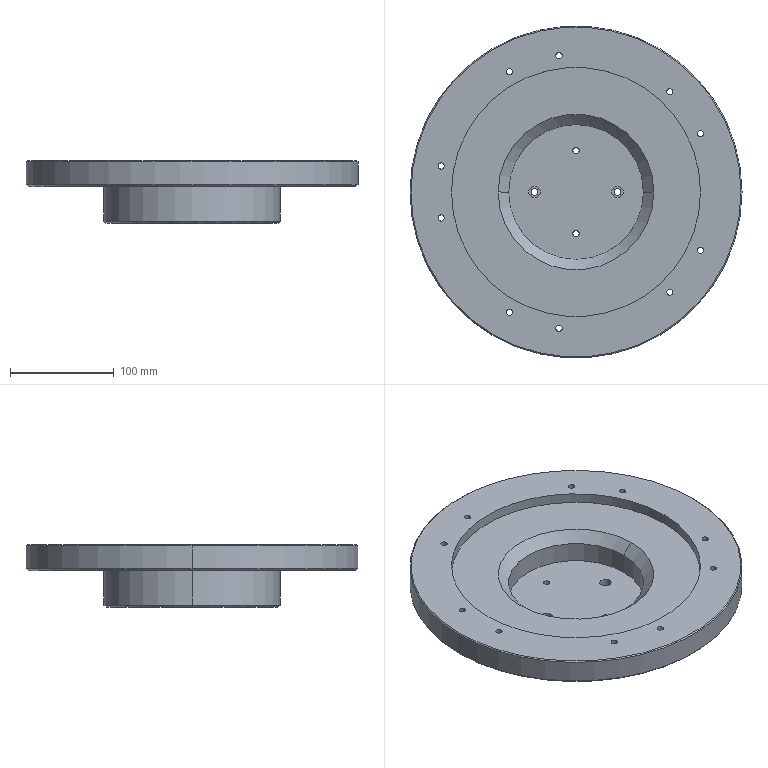NC program | NX | posted with a generic post | part box 320 x 320 x 60 mm
Lines 6415 to 7329 of 10816:
(ADAPTIVE_MILLING , TOOL : D10)
N12822 T10 M6
N12824 G54
N12826 G17 G0 G90 X-4.521 Y0.428 S7000 M3
N12828 G43 Z90. H10
N12830 Z63.
N12832 G94 G3 X-4.521 Y0.428 Z62.506 I4.5 J-0.048 F1000.
N12834 X-4.521 Y0.428 Z62.013 I4.5 J-0.048
N12836 X-4.521 Y0.428 Z61.519 I4.5 J-0.048
N12838 X-4.521 Y0.428 Z61.026 I4.5 J-0.048
N12840 X-4.521 Y0.428 Z60.532 I4.5 J-0.048
N12842 X-4.521 Y0.428 Z60.039 I4.5 J-0.048
N12844 X-4.521 Y0.428 Z59.545 I4.5 J-0.048
N12846 X-4.521 Y0.428 Z59.052 I4.5 J-0.048
N12848 X-4.521 Y0.428 Z58.558 I4.5 J-0.048
N12850 X-4.521 Y0.428 Z58.065 I4.5 J-0.048
N12852 X-4.521 Y0.428 Z57.571 I4.5 J-0.048
N12854 X-4.521 Y0.428 Z57.078 I4.5 J-0.048
N12856 X-4.521 Y0.428 Z56.584 I4.5 J-0.048
N12858 X-4.521 Y0.428 Z56.091 I4.5 J-0.048
N12860 X-4.521 Y0.428 Z55.597 I4.5 J-0.048
N12862 X-4.521 Y0.428 Z55.104 I4.5 J-0.048
N12864 X-4.521 Y0.428 Z54.61 I4.5 J-0.048
N12866 X-4.521 Y0.428 Z54.116 I4.5 J-0.048
N12868 X-4.521 Y0.428 Z53.623 I4.5 J-0.048
N12870 X-4.521 Y0.428 Z53.129 I4.5 J-0.048
N12872 X-4.521 Y0.428 Z52.636 I4.5 J-0.048
N12874 X-4.521 Y0.428 Z52.142 I4.5 J-0.048
N12876 X-4.521 Y0.428 Z51.649 I4.5 J-0.048
N12878 X-4.521 Y0.428 Z51.155 I4.5 J-0.048
N12880 X-4.521 Y0.428 Z50.662 I4.5 J-0.048
N12882 X-4.521 Y0.428 Z50.168 I4.5 J-0.048
N12884 X-4.521 Y0.428 Z49.675 I4.5 J-0.048
N12886 X-4.521 Y0.428 Z49.181 I4.5 J-0.048
N12888 X-4.521 Y0.428 Z48.688 I4.5 J-0.048
N12890 X-4.521 Y0.428 Z48.194 I4.5 J-0.048
N12892 X-4.521 Y0.428 Z47.701 I4.5 J-0.048
N12894 X-4.521 Y0.428 Z47.207 I4.5 J-0.048
N12896 X-4.521 Y0.428 Z46.713 I4.5 J-0.048
N12898 X-4.521 Y0.428 Z46.22 I4.5 J-0.048
N12900 X-4.521 Y0.428 Z45.726 I4.5 J-0.048
N12902 X-4.521 Y0.428 Z45.233 I4.5 J-0.048
N12904 X-4.521 Y0.428 Z44.739 I4.5 J-0.048
N12906 X-4.521 Y0.428 Z44.246 I4.5 J-0.048
N12908 X-4.521 Y0.428 Z43.752 I4.5 J-0.048
N12910 X-4.521 Y0.428 Z43.259 I4.5 J-0.048
N12912 X-4.521 Y0.428 Z42.765 I4.5 J-0.048
N12914 X-4.521 Y0.428 Z42.272 I4.5 J-0.048
N12916 X-4.521 Y0.428 Z41.778 I4.5 J-0.048
N12918 X-4.521 Y0.428 Z41.285 I4.5 J-0.048
N12920 X-4.521 Y0.428 Z40.791 I4.5 J-0.048
N12922 X-4.521 Y0.428 Z40.298 I4.5 J-0.048
N12924 X4.479 Y0.38 Z40.05 R-4.5
N12926 X3.82 Y-1.973 R-4.5 F3000.
N12928 X-1.968 Y4.837 R4.639
N12930 X4.067 Y-2.31 R-4.873
N12932 X-2.692 Y4.89 R5.04
N12934 X4.152 Y-2.848 R-5.255
N12936 X-2.938 Y5.204 R5.439
N12938 X4.261 Y-3.338 R-5.651
N12940 X-3.265 Y5.479 R5.843
N12942 X4.652 Y-3.527 R-6.063
N12944 X-3.679 Y5.714 R6.267
N12946 X4.876 Y-3.924 R-6.49
N12948 X-4.47 Y5.657 R6.705
N12950 X4.905 Y-4.534 R-6.929
N12952 X-4.472 Y6.225 R7.148
N12954 X4.687 Y-5.33 R-7.373
N12956 X-4.543 Y6.738 R7.599
N12958 X4.821 Y-5.82 R-7.834
N12960 X-4.706 Y7.2 R8.069
N12962 X5.046 Y-6.245 R-8.307
N12964 X-4.976 Y7.594 R8.545
N12966 X4.692 Y-7.072 R8.785
N12968 X-5.37 Y7.913 R-9.03
N12970 X4.783 Y-7.595 R9.275
N12972 X-4.799 Y8.871 R9.526
N12974 X5.388 Y-7.816 R-9.781
N12976 X-5.099 Y9.284 R10.034
N12978 X4.603 Y-8.849 R10.287
N12980 X9.365 Y5.283 R10.545
N12982 X-4.761 Y10.048 R10.545
N12984 X5.168 Y-9.148 R-10.808
N12986 X9.658 Y5.853 R11.072
N12988 X-5.428 Y10.296 R11.072
N12990 X4.668 Y-9.983 R11.335
N12992 X-5.024 Y11.099 R-11.602
N12994 X5.231 Y-10.315 R-11.872
N12996 X-4.809 Y11.788 R12.142
N12998 X5.143 Y-10.959 R-12.416
N13000 X-4.347 Y12.551 R12.687
N13002 X-12.216 Y-4.004 R12.961
N13004 X4.349 Y-11.869 R12.961
N13006 X-3.631 Y13.36 R13.238
N13008 X3.778 Y-12.638 R-13.517
N13010 X-3.169 Y14.056 R13.797
N13012 X2.962 Y-13.426 R14.079
N13014 X-1.944 Y14.847 R14.359
N13016 X1.364 Y-14.243 R14.641
N13018 X-1.015 Y15.515 R14.929
N13020 X1.708 Y-14.789 R-15.218
N13022 X-0.991 Y16.1 R15.509
N13024 X1.897 Y-15.357 R-15.802
N13026 X-0.804 Y16.698 R16.095
N13028 X1.369 Y-16.001 R-16.388
N13030 X0.7 Y17.285 R16.681
N13032 X-0.486 Y-16.642 R-16.974
N13034 X5.258 Y17.05 R17.262
N13036 X-8.144 Y-15.249 R17.546
N13038 X13.323 Y12.459 R17.822
N13040 X-17.648 Y-4.136 R18.078
N13042 X18.299 Y-1.668 R18.33
N13044 X-17.296 Y7.776 R18.599
N13046 X15.112 Y-11.032 R18.88
N13048 X-12.816 Y14.961 R19.171
N13050 X10.914 Y-15.801 R19.467
N13052 X-8.591 Y18.448 R19.762
N13054 X4.751 Y-19.151 R20.055
N13056 X4.115 Y20.505 R20.332
N13058 X-16.001 Y-12.72 R20.587
N13060 X19.972 Y6.714 R20.835
N13062 X-21.181 Y2.485 R21.098
N13064 X20.855 Y-4.74 R21.383
N13066 X-19.537 Y10.29 R21.682
N13068 X16.226 Y-14.545 R21.983
N13070 X-17.929 Y14.024 R-22.29
N13072 X9.392 Y-20.221 R22.596
N13074 X-4.289 Y23.088 R22.88
N13076 X-5.147 Y-22.255 R23.157
N13078 X21.34 Y10.206 R23.38
N13080 X-23.631 Y3.347 R23.625
N13082 X23.955 Y-1.628 R-23.927
N13084 X-23.567 Y6.887 R24.237
N13086 X22.582 Y-9.49 R24.55
N13088 X-24.014 Y7.657 R-24.872
N13090 X19.764 Y-15.358 R25.188
N13092 X-22.461 Y12.937 R-25.501
N13094 X4.511 Y-25.059 R25.803
N13096 X18.242 Y19.095 R26.017
N13098 X-26.403 Y0.385 R26.227
N13100 X26.625 Y1.599 R-26.527
N13102 X-26.485 Y5.882 R26.844
N13104 X26.595 Y-5.676 R27.163
N13106 X-26.735 Y7.632 R27.487
N13108 X26.727 Y-7.711 R27.814
N13110 X-27.877 Y5.589 R-28.144
N13112 X28.184 Y-4.483 R-28.48
N13114 X4.744 Y28.843 R28.81
N13116 X-28.559 Y5.535 R28.81
N13118 X28.672 Y-5.455 R29.14
N13120 X-28.981 Y6.784 R29.469
N13122 X28.998 Y-6.978 R29.799
N13124 X-29.762 Y6.307 R-30.133
N13126 X30.323 Y-3.706 R-30.47
N13128 X-30.799 Y4.012 R-30.805
N13130 X31.277 Y-0.047 R-31.144
N13132 X-31.668 Y1.376 R31.482
N13134 X31.935 Y1.583 R-31.819
N13136 X-32.057 Y-4.009 R-32.16
N13138 X32.486 Y3.539 R32.498
N13140 X-32.6 Y-4.942 R-32.837
N13142 X32.993 Y5.029 R33.176
N13144 X-32.883 Y-7.01 R-33.514
N13146 X33.838 Y3.603 R33.85
N13148 X-33.573 Y-7.015 R-34.188
N13150 X34.543 Y3.325 R34.526
N13152 X-34.656 Y-4.905 R-34.864
N13154 X35.278 Y2.571 R35.203
N13156 X-35.472 Y-3.949 R-35.542
N13158 X36.008 Y1.343 R35.88
N13160 X-36.3 Y-2.521 R-36.22
N13162 X36.691 Y1.359 R36.561
N13164 X-37.05 Y-1.478 R-36.901
N13166 X37.382 Y0.075 R37.241
N13168 X-37.779 Y0.015 R-37.583
N13170 X38.048 Y1.834 R-37.928
N13172 X-37.95 Y-5.909 R-38.274
N13174 X38.714 Y2.331 R38.617
N13176 X-38.85 Y-4.498 R-38.961
N13178 X39.399 Y2.436 R39.305
N13180 X-39.294 Y-6.201 R-39.65
N13182 X40.129 Y1.256 R39.992
N13184 X-40.379 Y-3.092 R-40.335
N13186 X40.792 Y-1.227 R40.678
N13188 X-41.181 Y-1.347 R-41.022
N13190 X41.477 Y-1.385 R41.367
N13192 X-41.844 Y-1.953 R-41.714
N13194 X41.778 Y-5.557 R42.056
N13196 X-39.998 Y15.006 R42.391
N13198 X40.52 Y-13.621 R-42.729
N13200 X-21.155 Y38.068 R43.058
N13202 X-29.201 Y-31.666 R43.28
N13204 X40.687 Y16.207 R43.509
N13206 X-16.027 Y41.228 R43.832
N13208 X-41.058 Y-15.458 R43.832
N13210 X44.284 Y-0.84 R44.157
N13212 X-44.383 Y5.578 R44.492
N13214 X43.714 Y-10.184 R44.831
N13216 X-29.833 Y34.518 R45.162
N13218 X13.629 Y-43.091 R45.449
N13220 X5.413 Y45.962 R45.735
N13222 X-41.372 Y-19.997 R45.98
N13224 X46.369 Y2.249 R46.266
N13226 X-46.508 Y-4.709 R-46.598
N13228 X45.415 Y-11.995 R46.931
N13230 X-32.54 Y34.902 R47.261
N13232 X20.494 Y-42.666 R47.56
N13234 X0.876 Y48.399 R47.856
N13236 X-43.015 Y-21.428 R48.1
N13238 X48.488 Y1.955 R48.374
N13240 X-1.73 Y49.096 R48.704
N13242 X-48.87 Y-1.141 R48.704
N13244 X46.63 Y-15.238 R49.038
N13246 X-32.794 Y37.52 R49.366
N13248 X18.056 Y-46.016 R49.669
N13250 X4.429 Y50.313 R49.963
N13252 X-46.063 Y-19.928 R50.212
N13254 X50.621 Y1.429 R50.49
N13256 X-50.879 Y-3.303 R-50.823
N13258 X48.682 Y-15.792 R51.157
N13260 X-35.221 Y38.182 R51.486
N13262 X26.537 Y-44.252 R51.798
N13264 X-4.165 Y52.49 R52.105
N13266 X-45.509 Y-25.746 R52.354
N13268 X52.037 Y9.189 R52.629
N13270 X-52.793 Y-5.732 R52.96
N13272 X51.698 Y-13.143 R53.294
N13274 X-49.071 Y22.497 R53.63
N13276 X45.234 Y-29.312 R53.969
N13278 X-26.916 Y47.74 R54.296
N13280 X-15.618 Y-52.027 R54.575
N13282 X39.989 Y38.126 R54.843
N13284 X-53.417 Y-13.915 R55.136
N13286 X54.84 Y-8.683 R55.443
N13288 X-53.239 Y17.64 R55.774
N13290 X46.293 Y-31.561 R56.108
N13292 X-24.252 Y51.52 R56.426
N13294 X-24.475 Y-50.883 R56.693
N13296 X43.64 Y37.235 R56.968
N13298 X-55.654 Y-13.824 R57.273
N13300 X57.468 Y-5.153 R57.589
N13302 X-58.015 Y3.899 R-57.928
N13304 X53.699 Y-22.607 R58.269
N13306 X-37.215 Y45.877 R58.6
N13308 X22.99 Y-54.002 R58.912
N13310 X5.6 Y59.496 R59.217
N13312 X-38.901 Y45.398 R59.436
N13314 X-51.45 Y-29.766 R59.483
N13316 X59.902 Y-0.131 R59.769
N13318 G1 X59.906 Y0.159
N13320 X59.727 Y4.699
N13322 X59.721 Y4.782
N13324 X59.163 Y9.44
N13326 X59.15 Y9.523
N13328 X58.224 Y14.122
N13330 X58.204 Y14.203
N13332 X56.914 Y18.714
N13334 X56.888 Y18.793
N13336 X55.243 Y23.187
N13338 X55.21 Y23.264
N13340 X53.221 Y27.513
N13342 X53.182 Y27.587
N13344 X50.861 Y31.664
N13346 X50.816 Y31.735
N13348 X48.177 Y35.614
N13350 X48.128 Y35.681
N13352 X45.188 Y39.338
N13354 X45.133 Y39.401
N13356 X41.912 Y42.811
N13358 X41.852 Y42.87
N13360 X38.369 Y46.013
N13362 X38.305 Y46.067
N13364 X34.583 Y48.923
N13366 X34.514 Y48.971
N13368 X30.577 Y51.522
N13370 X30.505 Y51.564
N13372 X26.377 Y53.793
N13374 X26.301 Y53.83
N13376 X22.009 Y55.723
N13378 X21.931 Y55.754
N13380 X17.501 Y57.299
N13382 X17.421 Y57.323
N13384 X12.882 Y58.51
N13386 X12.801 Y58.528
N13388 X8.182 Y59.35
N13390 X8.098 Y59.362
N13392 X3.335 Y59.819
N13394 X3.249 Y59.823
N13396 X-1.55 Y59.892
N13398 X-1.62 Y59.89
N13400 X-6.395 Y59.569
N13402 X-6.48 Y59.56
N13404 X-11.212 Y58.853
N13406 X-11.296 Y58.837
N13408 X-15.955 Y57.748
N13410 X-16.038 Y57.725
N13412 X-20.593 Y56.261
N13414 X-20.673 Y56.232
N13416 X-25.095 Y54.403
N13418 X-25.173 Y54.367
N13420 X-29.431 Y52.184
N13422 X-29.505 Y52.143
N13424 X-33.573 Y49.622
N13426 X-33.643 Y49.574
N13428 X-37.492 Y46.731
N13430 X-37.559 Y46.677
N13432 X-41.164 Y43.531
N13434 X-41.226 Y43.472
N13436 X-44.564 Y40.044
N13438 X-44.621 Y39.98
N13440 X-47.669 Y36.292
N13442 X-47.721 Y36.224
N13444 X-50.459 Y32.3
N13446 X-50.505 Y32.228
N13448 X-52.916 Y28.094
N13450 X-52.956 Y28.019
N13452 X-55.023 Y23.703
N13454 X-55.057 Y23.625
N13456 X-56.767 Y19.156
N13458 X-56.794 Y19.075
N13460 X-58.135 Y14.482
N13462 X-58.156 Y14.399
N13464 X-59.119 Y9.712
N13466 X-59.133 Y9.628
N13468 X-59.713 Y4.878
N13470 X-59.72 Y4.793
N13472 X-59.912 Y0.011
N13474 X-59.913 Y-0.031
N13476 X-59.912 Y-0.073
N13478 X-59.727 Y-4.706
N13480 X-59.72 Y-4.789
N13482 X-59.171 Y-9.393
N13484 X-59.158 Y-9.475
N13486 X-58.248 Y-14.022
N13488 X-58.228 Y-14.102
N13490 X-56.963 Y-18.564
N13492 X-56.938 Y-18.642
N13494 X-55.325 Y-22.99
N13496 X-55.293 Y-23.067
N13498 X-53.344 Y-27.274
N13500 X-53.306 Y-27.348
N13502 X-51.031 Y-31.388
N13504 X-50.987 Y-31.459
N13506 X-48.335 Y-35.4
N13508 X-48.285 Y-35.468
N13510 X-45.324 Y-39.181
N13512 X-45.268 Y-39.245
N13514 X-42.018 Y-42.708
N13516 X-41.957 Y-42.767
N13518 X-38.438 Y-45.956
N13520 X-38.373 Y-46.01
N13522 X-34.608 Y-48.905
N13524 X-34.539 Y-48.954
N13526 X-30.552 Y-51.536
N13528 X-30.48 Y-51.579
N13530 X-26.298 Y-53.831
N13532 X-26.222 Y-53.868
N13534 X-21.873 Y-55.776
N13536 X-21.794 Y-55.807
N13538 X-17.305 Y-57.358
N13540 X-17.224 Y-57.382
N13542 X-12.625 Y-58.566
N13544 X-12.542 Y-58.584
N13546 X-7.862 Y-59.394
N13548 X-7.778 Y-59.405
N13550 X-3.048 Y-59.834
N13552 X-2.964 Y-59.838
N13554 X1.796 Y-59.885
N13556 X1.87 Y-59.883
N13558 X6.608 Y-59.546
N13560 X6.692 Y-59.537
N13562 X11.387 Y-58.82
N13564 X11.47 Y-58.804
N13566 X16.092 Y-57.71
N13568 X16.173 Y-57.687
N13570 X20.692 Y-56.225
N13572 X20.771 Y-56.196
N13574 X25.157 Y-54.374
N13576 X25.234 Y-54.338
N13578 X29.459 Y-52.169
N13580 X29.533 Y-52.127
N13582 X33.569 Y-49.624
N13584 X33.639 Y-49.577
N13586 X37.46 Y-46.756
N13588 X37.526 Y-46.703
N13590 X41.108 Y-43.584
N13592 X41.169 Y-43.526
N13594 X44.487 Y-40.128
N13596 X44.544 Y-40.065
N13598 X47.578 Y-36.411
N13600 X47.629 Y-36.344
N13602 X50.358 Y-32.457
N13604 X50.404 Y-32.386
N13606 X52.836 Y-28.244
N13608 X52.877 Y-28.169
N13610 X54.963 Y-23.843
N13612 X54.997 Y-23.764
N13614 X56.724 Y-19.283
N13616 X56.751 Y-19.202
N13618 X58.107 Y-14.594
N13620 X58.128 Y-14.511
N13622 X59.103 Y-9.809
N13624 X59.117 Y-9.724
N13626 X59.706 Y-4.958
N13628 X59.713 Y-4.872
N13630 X59.912 Y-0.074
N13632 X59.913 Y-0.03
N13634 X59.912 Y0.011
N13636 X59.904 Y0.211
N13638 G3 X58.72 Y1.166 R1.014
N13640 G1 X57.371 Y0.929
N13642 Z43.05
N13644 G0 Z90.
N13646 X-57.304 Y0.679
N13648 Z44.048
N13650 G1 Z41.048 F1000.
N13652 X-59.04 Y0.542 F3000.
N13654 G3 X-59.86 Y-0.006 R1.024
N13656 X-60.407 Y-2.773 R6.867
N13658 X-59.046 Y-13.96 R44.76
N13660 X47.926 Y-37.169 R60.65
N13662 X53.185 Y-29.142 R100.289
N13664 X-2.18 Y60.625 R60.62
N13666 X-60.621 Y2.622 R60.669
N13668 G1 X-60.649 Y2.323
N13670 X-60.679 Y2.024
N13672 X-60.724 Y1.627
N13674 X-60.759 Y1.329
N13676 X-60.843 Y0.634
N13678 X-60.9 Y0.143
N13680 X-60.904 Y0.022
N13682 X-60.905 Y-0.018
N13684 X-60.904 Y-0.061
N13686 X-60.711 Y-4.854
N13688 X-60.704 Y-4.937
N13690 X-60.127 Y-9.699
N13692 X-60.114 Y-9.782
N13694 X-59.158 Y-14.481
N13696 X-59.138 Y-14.563
N13698 X-57.808 Y-19.171
N13700 X-57.782 Y-19.251
N13702 X-56.088 Y-23.738
N13704 X-56.055 Y-23.815
N13706 X-54.007 Y-28.152
N13708 X-53.968 Y-28.227
N13710 X-51.58 Y-32.386
N13712 X-51.535 Y-32.457
N13714 X-48.8 Y-36.441
N13716 X-48.749 Y-36.509
N13718 X-45.701 Y-40.259
N13720 X-45.645 Y-40.322
N13722 X-42.305 Y-43.814
N13724 X-42.244 Y-43.873
N13726 X-38.632 Y-47.084
N13728 X-38.567 Y-47.138
N13730 X-34.708 Y-50.047
N13732 X-34.639 Y-50.095
N13734 X-30.558 Y-52.684
N13736 X-30.485 Y-52.726
N13738 X-26.209 Y-54.977
N13740 X-26.132 Y-55.013
N13742 X-21.688 Y-56.912
N13744 X-21.609 Y-56.942
N13746 X-17.027 Y-58.476
N13748 X-16.945 Y-58.5
N13750 X-12.254 Y-59.659
N13752 X-12.171 Y-59.676
N13754 X-7.402 Y-60.453
N13756 X-7.317 Y-60.463
N13758 X-2.501 Y-60.853
N13760 X-2.416 Y-60.856
N13762 X2.416
N13764 X2.501 Y-60.853
N13766 X7.317 Y-60.463
N13768 X7.402 Y-60.453
N13770 X12.171 Y-59.676
N13772 X12.254 Y-59.659
N13774 X16.945 Y-58.5
N13776 X17.027 Y-58.476
N13778 X21.609 Y-56.942
N13780 X21.688 Y-56.912
N13782 X26.132 Y-55.013
N13784 X26.209 Y-54.977
N13786 X30.485 Y-52.726
N13788 X30.558 Y-52.684
N13790 X34.639 Y-50.095
N13792 X34.708 Y-50.047
N13794 X38.567 Y-47.138
N13796 X38.632 Y-47.084
N13798 X42.244 Y-43.873
N13800 X42.305 Y-43.814
N13802 X45.645 Y-40.322
N13804 X45.701 Y-40.259
N13806 X48.749 Y-36.509
N13808 X48.8 Y-36.441
N13810 X51.535 Y-32.457
N13812 X51.58 Y-32.386
N13814 X53.968 Y-28.227
N13816 X54.007 Y-28.152
N13818 X56.055 Y-23.815
N13820 X56.088 Y-23.738
N13822 X57.782 Y-19.251
N13824 X57.808 Y-19.171
N13826 X59.138 Y-14.563
N13828 X59.158 Y-14.481
N13830 X60.114 Y-9.782
N13832 X60.127 Y-9.699
N13834 X60.704 Y-4.937
N13836 X60.711 Y-4.854
N13838 X60.904 Y-0.061
N13840 X60.905 Y-0.019
N13842 X60.904 Y0.023
N13844 X60.715 Y4.794
N13846 X60.709 Y4.878
N13848 X60.14 Y9.62
N13850 X60.127 Y9.702
N13852 X59.182 Y14.383
N13854 X59.162 Y14.465
N13856 X57.847 Y19.056
N13858 X57.82 Y19.135
N13860 X56.143 Y23.607
N13862 X56.111 Y23.684
N13864 X54.083 Y28.008
N13866 X54.044 Y28.082
N13868 X51.678 Y32.23
N13870 X51.633 Y32.301
N13872 X48.944 Y36.247
N13874 X48.894 Y36.315
N13876 X45.898 Y40.034
N13878 X45.843 Y40.097
N13880 X42.56 Y43.566
N13882 X42.5 Y43.624
N13884 X38.952 Y46.82
N13886 X38.887 Y46.874
N13888 X35.095 Y49.776
N13890 X35.026 Y49.825
N13892 X31.015 Y52.416
N13894 X30.943 Y52.458
N13896 X26.737 Y54.722
N13898 X26.662 Y54.758
N13900 X22.29 Y56.679
N13902 X22.212 Y56.71
N13904 X17.7 Y58.276
N13906 X17.62 Y58.3
N13908 X12.998 Y59.501
N13910 X12.916 Y59.519
N13912 X8.212 Y60.348
N13914 X8.13 Y60.359
N13916 X3.513 Y60.803
N13918 X3.432 Y60.808
N13920 X-1.226 Y60.893
N13922 X-1.289 Y60.891
N13924 X-5.92 Y60.616
N13926 X-6.001 Y60.608
N13928 X-10.597 Y59.976
N13930 X-10.677 Y59.961
N13932 X-15.211 Y58.975
N13934 X-15.289 Y58.954
N13936 X-19.733 Y57.619
N13938 X-19.81 Y57.593
N13940 X-24.136 Y55.918
N13942 X-24.211 Y55.886
N13944 X-28.395 Y53.88
N13946 X-28.467 Y53.842
N13948 X-32.483 Y51.519
N13950 X-32.551 Y51.476
N13952 X-36.375 Y48.849
N13954 X-36.441 Y48.8
N13956 X-40.05 Y45.884
N13958 X-40.111 Y45.831
N13960 X-43.483 Y42.645
N13962 X-43.54 Y42.586
N13964 X-46.656 Y39.149
N13966 X-46.708 Y39.086
N13968 X-49.548 Y35.417
N13970 X-49.595 Y35.351
N13972 X-52.142 Y31.473
N13974 X-52.184 Y31.404
N13976 X-54.423 Y27.34
N13978 X-54.46 Y27.267
N13980 X-56.377 Y23.043
N13982 X-56.408 Y22.967
N13984 X-57.993 Y18.607
N13986 X-58.017 Y18.529
N13988 X-59.26 Y14.059
N13990 X-59.278 Y13.98
N13992 X-60.17 Y9.427
N13994 X-60.183 Y9.347
N13996 X-60.72 Y4.738
N13998 X-60.726 Y4.657
N14000 X-60.903 Y0.061
N14002 G3 X-59.75 Y-0.978 R1.013
N14004 G1 X-58.215 Y-0.758
N14006 Z44.048
N14008 G0 Z90.
N14010 X-58.296 Y0.616
N14012 Z45.045
N14014 G1 Z42.045 F1000.
N14016 X-60.032 Y0.479 F3000.
N14018 G3 X-60.853 Y-0.069 R1.024
N14020 X-61.398 Y-2.837 R6.894
N14022 X-60.002 Y-14.221 R45.657
N14024 X48.961 Y-37.465 R61.653
N14026 X54.412 Y-28.968 R96.299
N14028 X-45.084 Y42.067 R61.648
N14030 X-61.624 Y2.497 R61.743
N14032 G1 X-61.651 Y2.199
N14034 X-61.693 Y1.801
N14036 X-61.738 Y1.403
N14038 X-61.844 Y0.51
N14040 X-61.879 Y0.212
N14042 X-61.902 Y-0.003
N14044 X-61.903 Y-0.03
N14046 X-61.902 Y-0.072
N14048 X-61.711 Y-4.855
N14050 X-61.705 Y-4.938
N14052 X-61.139 Y-9.691
N14054 X-61.126 Y-9.772
N14056 X-60.188 Y-14.466
N14058 X-60.169 Y-14.546
N14060 X-58.865 Y-19.152
N14062 X-58.839 Y-19.23
N14064 X-57.177 Y-23.719
N14066 X-57.146 Y-23.795
N14068 X-55.136 Y-28.14
N14070 X-55.099 Y-28.213
N14072 X-52.754 Y-32.386
N14074 X-52.711 Y-32.457
N14076 X-50.07 Y-36.399
N14078 X-50.021 Y-36.465
N14080 X-47.081 Y-40.19
N14082 X-47.028 Y-40.252
N14084 X-43.806 Y-43.737
N14086 X-43.748 Y-43.794
N14088 X-40.265 Y-47.017
N14090 X-40.202 Y-47.07
N14092 X-36.478 Y-50.012
N14094 X-36.412 Y-50.06
N14096 X-32.47 Y-52.702
N14098 X-32.401 Y-52.745
N14100 X-28.265 Y-55.072
N14102 X-28.192 Y-55.11
N14104 X-23.887 Y-57.107
N14106 X-23.812 Y-57.139
N14108 X-19.365 Y-58.795
N14110 X-19.287 Y-58.821
N14112 X-14.724 Y-60.125
N14114 X-14.645 Y-60.145
N14116 X-9.994 Y-61.09
N14118 X-9.913 Y-61.103
N14120 X-5.203 Y-61.683
N14122 X-5.122 Y-61.69
N14124 X-0.381 Y-61.901
N14126 X-0.334 Y-61.902
N14128 X-0.299 Y-61.901
N14130 X4.444 Y-61.742
N14132 X4.526 Y-61.736
N14134 X9.242 Y-61.208
N14136 X9.323 Y-61.196
N14138 X13.983 Y-60.302
N14140 X14.063 Y-60.283
N14142 X18.64 Y-59.029
N14144 X18.718 Y-59.004
N14146 X23.183 Y-57.397
N14148 X23.259 Y-57.366
N14150 X27.585 Y-55.416
N14152 X27.658 Y-55.379
N14154 X31.819 Y-53.098
N14156 X31.89 Y-53.056
N14158 X35.86 Y-50.457
N14160 X35.927 Y-50.409
N14162 X39.683 Y-47.509
N14164 X39.746 Y-47.456
N14166 X43.265 Y-44.272
N14168 X43.323 Y-44.215
N14170 X46.583 Y-40.766
N14172 X46.637 Y-40.705
N14174 X49.618 Y-37.012
N14176 X49.667 Y-36.947
N14178 X52.352 Y-33.032
N14180 X52.394 Y-32.966
N14182 G3 X58.136 Y-21.262 R66.838
N14184 X61.3 Y-8.613 R66.851
N14186 X61.902 Y0.071 R71.698
N14188 G1 X61.706 Y4.925
N14190 X61.699 Y5.009
N14192 X61.116 Y9.83
N14194 X61.103 Y9.913
N14196 X60.138 Y14.672
N14198 X60.118 Y14.753
N14200 X58.777 Y19.421
N14202 X58.75 Y19.5
N14204 X57.041 Y24.046
N14206 X57.008 Y24.123
N14208 X54.942 Y28.517
N14210 X54.903 Y28.592
N14212 X52.493 Y32.808
N14214 X52.449 Y32.879
N14216 X49.71 Y36.889
N14218 X49.66 Y36.956
N14220 X46.61 Y40.735
N14222 X46.555 Y40.798
N14224 X43.213 Y44.322
N14226 X43.153 Y44.381
N14228 X39.542 Y47.627
N14230 X39.477 Y47.68
N14232 X35.618 Y50.628
N14234 X35.549 Y50.676
N14236 X31.468 Y53.307
N14238 X31.395 Y53.35
N14240 X27.117 Y55.646
N14242 X27.041 Y55.683
N14244 X22.593 Y57.632
N14246 X22.515 Y57.662
N14248 X17.926 Y59.25
N14250 X17.846 Y59.274
N14252 X13.144 Y60.49
N14254 X13.062 Y60.508
N14256 X8.278 Y61.346
N14258 X8.197 Y61.357
N14260 X3.504 Y61.803
N14262 X3.423 Y61.807
N14264 X-1.309 Y61.889
N14266 X-1.372 Y61.887
N14268 X-6.078 Y61.603
N14270 X-6.159 Y61.595
N14272 X-10.828 Y60.948
N14274 X-10.908 Y60.933
N14276 X-15.514 Y59.926
N14278 X-15.593 Y59.906
N14280 X-20.106 Y58.546
N14282 X-20.183 Y58.519
N14284 X-24.578 Y56.813
N14286 X-24.653 Y56.781
N14288 X-28.902 Y54.74
N14290 X-28.974 Y54.702
N14292 X-33.053 Y52.339
N14294 X-33.122 Y52.295
N14296 X-37.006 Y49.623
N14298 X-37.071 Y49.574
N14300 X-40.736 Y46.609
N14302 X-40.797 Y46.556
N14304 X-44.222 Y43.316
N14306 X-44.279 Y43.258
N14308 X-47.442 Y39.763
N14310 X-47.495 Y39.7
N14312 X-50.378 Y35.971
N14314 X-50.425 Y35.905
N14316 X-53.012 Y31.963
N14318 X-53.054 Y31.893
N14320 X-55.327 Y27.763
N14322 X-55.363 Y27.691
N14324 X-57.31 Y23.397
N14326 X-57.341 Y23.322
N14328 X-58.949 Y18.89
N14330 X-58.974 Y18.813
N14332 X-60.235 Y14.27
N14334 X-60.253 Y14.191
N14336 X-61.159 Y9.565
N14338 X-61.171 Y9.484
N14340 X-61.716 Y4.801
N14342 X-61.722 Y4.72
N14344 X-61.902 Y0.01
N14346 X-61.903 Y-0.03
N14348 G3 X-60.988 Y-1.016 R1.015
N14350 G1 X-59.213 Y-1.183
N14352 Z45.045
N14354 G0 Z90.
N14356 X-59.294 Y0.628
N14358 Z46.043
N14360 G1 Z43.043 F1000.
N14362 X-61.03 Y0.492 F3000.
N14364 G3 X-61.851 Y-0.057 R1.024
N14366 X-62.398 Y-2.824 R6.916
N14368 X-61.075 Y-14.017 R45.822
N14370 X-62.603 Y2.803 R-62.665
N14372 G1 X-62.618 Y2.603
N14374 X-62.645 Y2.304
N14376 X-62.675 Y2.006
N14378 X-62.729 Y1.509
N14380 X-62.858 Y0.416
N14382 X-62.898 Y0.064
N14384 X-62.9 Y-0.021
N14386 Y-0.058
N14388 G3 X-61.507 Y-13.163 R67.934
N14390 X-57.413 Y-25.692 R67.946
N14392 X-53.267 Y-33.452 R72.886
N14394 G1 X-50.551 Y-37.429
N14396 X-50.503 Y-37.494
N14398 X-47.488 Y-41.246
N14400 X-47.434 Y-41.308
N14402 X-44.137 Y-44.814
N14404 X-44.078 Y-44.871
N14406 X-40.518 Y-48.11
N14408 X-40.456 Y-48.163
N14410 X-36.655 Y-51.115
N14412 X-36.588 Y-51.163
N14414 X-32.569 Y-53.811
N14416 X-32.499 Y-53.853
N14418 X-28.286 Y-56.181
N14420 X-28.213 Y-56.217
N14422 X-23.832 Y-58.21
N14424 X-23.756 Y-58.241
N14426 X-19.233 Y-59.887
N14428 X-19.155 Y-59.912
N14430 X-14.518 Y-61.201
N14432 X-14.438 Y-61.22
N14434 X-9.715 Y-62.145
N14436 X-9.634 Y-62.157
N14438 X-4.853 Y-62.712
N14440 X-4.772 Y-62.718
N14442 X0.038 Y-62.899
N14444 X0.078 Y-62.9
N14446 X0.12 Y-62.899
N14448 X4.929 Y-62.706
N14450 X5.011 Y-62.7
N14452 X9.79 Y-62.133
N14454 X9.871 Y-62.12
N14456 X14.592 Y-61.183
N14458 X14.672 Y-61.164
N14460 X19.306 Y-59.864
N14462 X19.383 Y-59.838
N14464 X23.902 Y-58.181
N14466 X23.978 Y-58.15
N14468 X28.354 Y-56.146
N14470 X28.427 Y-56.109
N14472 X32.634 Y-53.771
N14474 X32.704 Y-53.729
N14476 X36.716 Y-51.071
N14478 X36.783 Y-51.023
N14480 X40.577 Y-48.061
N14482 X40.639 Y-48.009
N14484 X44.191 Y-44.761
N14486 X44.249 Y-44.703
N14488 X47.538 Y-41.189
N14490 X47.591 Y-41.127
N14492 X50.597 Y-37.367
N14494 X50.645 Y-37.302
N14496 X53.349 Y-33.32
N14498 X53.393 Y-33.25
N14500 X55.83 Y-28.972
N14502 X55.868 Y-28.898
N14504 X57.957 Y-24.44
N14506 X57.99 Y-24.363
N14508 X59.717 Y-19.753
N14510 X59.744 Y-19.674
N14512 X61.099 Y-14.941
N14514 X61.119 Y-14.86
N14516 X62.094 Y-10.034
N14518 X62.107 Y-9.952
N14520 X62.695 Y-5.064
N14522 X62.702 Y-4.98
N14524 X62.899 Y-0.06
N14526 X62.9 Y-0.018
N14528 Y0.021
N14530 X62.724 Y4.699
N14532 X62.718 Y4.779
N14534 X62.189 Y9.431
N14536 X62.177 Y9.509
N14538 X61.297 Y14.108
N14540 X61.279 Y14.186
N14542 X60.054 Y18.705
N14544 X60.03 Y18.781
N14546 X58.467 Y23.194
N14548 X58.438 Y23.268
N14550 X56.545 Y27.551
N14552 X56.51 Y27.622
N14554 X54.298 Y31.75
N14556 X54.258 Y31.818
N14558 X51.741 Y35.766
N14560 X51.696 Y35.832
N14562 X48.887 Y39.578
N14564 X48.837 Y39.64
N14566 X45.753 Y43.163
N14568 X45.698 Y43.221
N14570 X42.357 Y46.5
N14572 X42.298 Y46.554
N14574 X38.717 Y49.571
N14576 X38.655 Y49.62
N14578 X34.856 Y52.358
N14580 X34.79 Y52.402
N14582 X30.796 Y54.845
N14584 X30.726 Y54.884
N14586 X26.558 Y57.018
N14588 X26.486 Y57.051
N14590 X22.169 Y58.863
N14592 X22.095 Y58.891
N14594 X17.653 Y60.372
N14596 X17.576 Y60.394
N14598 X13.035 Y61.534
N14600 X12.957 Y61.551
N14602 X8.343 Y62.344
N14604 X8.263 Y62.354
N14606 X3.496 Y62.802
N14608 X3.415 Y62.807
N14610 X-1.39 Y62.885
N14612 X-1.454 Y62.883
N14614 X-6.233 Y62.59
N14616 X-6.314 Y62.582
N14618 X-11.056 Y61.92
N14620 X-11.136 Y61.906
N14622 X-15.813 Y60.879
N14624 X-15.891 Y60.859
N14626 X-20.475 Y59.474
N14628 X-20.551 Y59.447
N14630 X-25.014 Y57.712
N14632 X-25.088 Y57.68
N14634 X-29.403 Y55.604
N14636 X-29.475 Y55.566
N14638 X-33.616 Y53.163
N14640 X-33.685 Y53.12
N14642 X-37.628 Y50.403
N14644 X-37.693 Y50.355